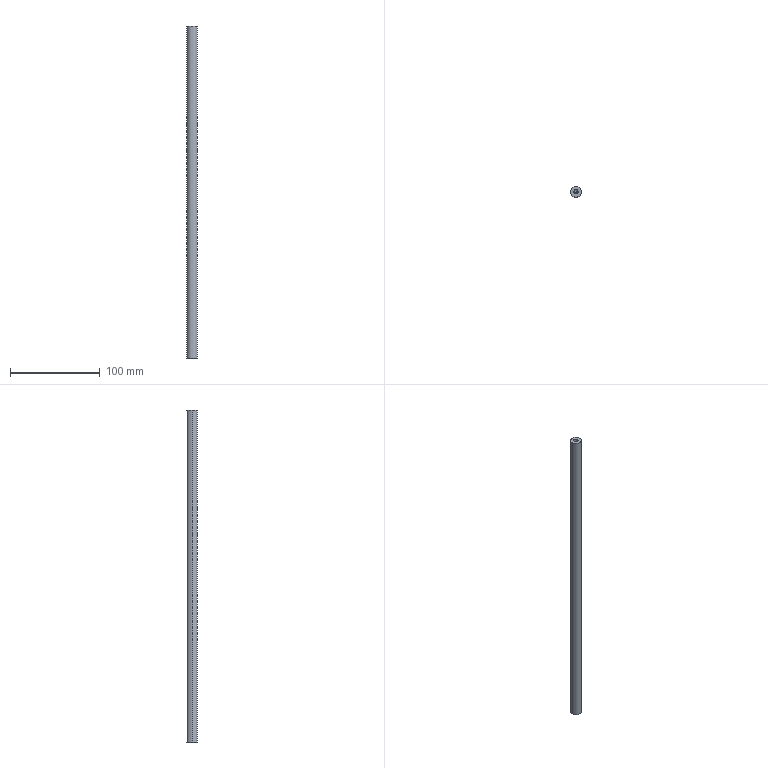Part | STEP file | 602-12-0049 | 1 solid | 12 faces | box 12 x 12 x 370 mm | volume 41119 mm3 | cylinder 6 | cone 4 | plane 2 | commonest cylinder face diameters 5 x4 12 x2
STEP:
#1=CARTESIAN_POINT('',(0.,0.,0.));
#2=DIRECTION('',(0.,0.,1.));
#3=DIRECTION('',(1.,0.,0.));
#4=AXIS2_PLACEMENT_3D('',#1,#2,#3);
#5=CARTESIAN_POINT('',(-2.5,0.,18.));
#6=VERTEX_POINT('',#5);
#7=CARTESIAN_POINT('',(-2.5,0.,0.));
#8=VERTEX_POINT('',#7);
#9=CARTESIAN_POINT('',(-2.5,0.,0.));
#10=DIRECTION('',(0.,0.,-1.));
#11=VECTOR('',#10,1.);
#12=LINE('',#9,#11);
#13=CARTESIAN_POINT('',(0.,0.,0.));
#14=DIRECTION('',(0.,0.,-1.));
#15=DIRECTION('',(-1.,0.,0.));
#16=AXIS2_PLACEMENT_3D('',#13,#14,#15);
#17=CYLINDRICAL_SURFACE('',#16,2.5);
#18=CARTESIAN_POINT('',(6.283,0.));
#19=DIRECTION('',(0.,1.));
#20=VECTOR('',#19,1.);
#21=LINE('',#18,#20);
#22=(GEOMETRIC_REPRESENTATION_CONTEXT(2)PARAMETRIC_REPRESENTATION_CONTEXT()REPRESENTATION_CONTEXT('',''));
#23=DEFINITIONAL_REPRESENTATION('',(#21),#22);
#24=PCURVE('',#17,#23);
#25=CARTESIAN_POINT('',(0.,0.,0.));
#26=DIRECTION('',(0.,0.,-1.));
#27=DIRECTION('',(-1.,0.,0.));
#28=AXIS2_PLACEMENT_3D('',#25,#26,#27);
#29=CYLINDRICAL_SURFACE('',#28,2.5);
#30=CARTESIAN_POINT('',(0.,0.));
#31=DIRECTION('',(0.,1.));
#32=VECTOR('',#31,1.);
#33=LINE('',#30,#32);
#34=(GEOMETRIC_REPRESENTATION_CONTEXT(2)PARAMETRIC_REPRESENTATION_CONTEXT()REPRESENTATION_CONTEXT('',''));
#35=DEFINITIONAL_REPRESENTATION('',(#33),#34);
#36=PCURVE('',#29,#35);
#37=SURFACE_CURVE('',#12,(#24,#36),.PCURVE_S1.);
#38=EDGE_CURVE('',#6,#8,#37,.T.);
#39=ORIENTED_EDGE('',*,*,#38,.T.);
#40=CARTESIAN_POINT('',(2.5,0.,0.));
#41=VERTEX_POINT('',#40);
#42=CARTESIAN_POINT('',(0.,0.,0.));
#43=DIRECTION('',(0.,0.,-1.));
#44=DIRECTION('',(-1.,0.,0.));
#45=AXIS2_PLACEMENT_3D('',#42,#43,#44);
#46=CIRCLE('',#45,2.5);
#47=CARTESIAN_POINT('',(0.,0.));
#48=DIRECTION('',(1.,0.));
#49=VECTOR('',#48,1.);
#50=LINE('',#47,#49);
#51=(GEOMETRIC_REPRESENTATION_CONTEXT(2)PARAMETRIC_REPRESENTATION_CONTEXT()REPRESENTATION_CONTEXT('',''));
#52=DEFINITIONAL_REPRESENTATION('',(#50),#51);
#53=PCURVE('',#17,#52);
#54=CARTESIAN_POINT('',(0.,0.,0.));
#55=DIRECTION('',(0.,0.,1.));
#56=DIRECTION('',(1.,0.,0.));
#57=AXIS2_PLACEMENT_3D('',#54,#55,#56);
#58=PLANE('',#57);
#59=CARTESIAN_POINT('',(-2.5,0.));
#60=CARTESIAN_POINT('',(-2.5,4.33));
#61=CARTESIAN_POINT('',(1.25,2.165));
#62=CARTESIAN_POINT('',(5.,0.));
#63=CARTESIAN_POINT('',(1.25,-2.165));
#64=CARTESIAN_POINT('',(-2.5,-4.33));
#65=CARTESIAN_POINT('',(-2.5,0.));
#66=(BOUNDED_CURVE()B_SPLINE_CURVE(2,(#59,#60,#61,#62,#63,#64,#65),.UNSPECIFIED.,.T.,.F.)B_SPLINE_CURVE_WITH_KNOTS((1,2,2,2,2,1),(-2.094,0.,2.094,4.189,6.283,8.378),.UNSPECIFIED.)CURVE()GEOMETRIC_REPRESENTATION_ITEM()RATIONAL_B_SPLINE_CURVE((1.,0.5,1.,0.5,1.,0.5,1.))REPRESENTATION_ITEM(''));
#67=(GEOMETRIC_REPRESENTATION_CONTEXT(2)PARAMETRIC_REPRESENTATION_CONTEXT()REPRESENTATION_CONTEXT('',''));
#68=DEFINITIONAL_REPRESENTATION('',(#66),#67);
#69=PCURVE('',#58,#68);
#70=SURFACE_CURVE('',#46,(#53,#69),.PCURVE_S1.);
#71=EDGE_CURVE('',#41,#8,#70,.T.);
#72=ORIENTED_EDGE('',*,*,#71,.F.);
#73=CARTESIAN_POINT('',(2.5,0.,18.));
#74=VERTEX_POINT('',#73);
#75=CARTESIAN_POINT('',(2.5,0.,0.));
#76=DIRECTION('',(0.,0.,-1.));
#77=VECTOR('',#76,1.);
#78=LINE('',#75,#77);
#79=CARTESIAN_POINT('',(3.142,0.));
#80=DIRECTION('',(0.,1.));
#81=VECTOR('',#80,1.);
#82=LINE('',#79,#81);
#83=(GEOMETRIC_REPRESENTATION_CONTEXT(2)PARAMETRIC_REPRESENTATION_CONTEXT()REPRESENTATION_CONTEXT('',''));
#84=DEFINITIONAL_REPRESENTATION('',(#82),#83);
#85=PCURVE('',#17,#84);
#86=CARTESIAN_POINT('',(3.142,0.));
#87=DIRECTION('',(0.,1.));
#88=VECTOR('',#87,1.);
#89=LINE('',#86,#88);
#90=(GEOMETRIC_REPRESENTATION_CONTEXT(2)PARAMETRIC_REPRESENTATION_CONTEXT()REPRESENTATION_CONTEXT('',''));
#91=DEFINITIONAL_REPRESENTATION('',(#89),#90);
#92=PCURVE('',#29,#91);
#93=SURFACE_CURVE('',#78,(#85,#92),.PCURVE_S1.);
#94=EDGE_CURVE('',#74,#41,#93,.T.);
#95=ORIENTED_EDGE('',*,*,#94,.F.);
#96=CARTESIAN_POINT('',(0.,0.,18.));
#97=DIRECTION('',(0.,0.,-1.));
#98=DIRECTION('',(-1.,0.,0.));
#99=AXIS2_PLACEMENT_3D('',#96,#97,#98);
#100=CIRCLE('',#99,2.5);
#101=CARTESIAN_POINT('',(0.,-18.));
#102=DIRECTION('',(1.,0.));
#103=VECTOR('',#102,1.);
#104=LINE('',#101,#103);
#105=(GEOMETRIC_REPRESENTATION_CONTEXT(2)PARAMETRIC_REPRESENTATION_CONTEXT()REPRESENTATION_CONTEXT('',''));
#106=DEFINITIONAL_REPRESENTATION('',(#104),#105);
#107=PCURVE('',#17,#106);
#108=CARTESIAN_POINT('',(0.,0.,18.));
#109=DIRECTION('',(0.,0.,-1.));
#110=DIRECTION('',(-1.,0.,0.));
#111=AXIS2_PLACEMENT_3D('',#108,#109,#110);
#112=CONICAL_SURFACE('',#111,2.5,1.03);
#113=CARTESIAN_POINT('',(0.,0.));
#114=DIRECTION('',(1.,0.));
#115=VECTOR('',#114,1.);
#116=LINE('',#113,#115);
#117=(GEOMETRIC_REPRESENTATION_CONTEXT(2)PARAMETRIC_REPRESENTATION_CONTEXT()REPRESENTATION_CONTEXT('',''));
#118=DEFINITIONAL_REPRESENTATION('',(#116),#117);
#119=PCURVE('',#112,#118);
#120=SURFACE_CURVE('',#100,(#107,#119),.PCURVE_S1.);
#121=EDGE_CURVE('',#74,#6,#120,.T.);
#122=ORIENTED_EDGE('',*,*,#121,.T.);
#123=EDGE_LOOP('',(#39,#72,#95,#122));
#124=FACE_BOUND('',#123,.F.);
#125=ADVANCED_FACE('',(#124),#17,.F.);
#126=ORIENTED_EDGE('',*,*,#121,.F.);
#127=CARTESIAN_POINT('',(0.,0.,19.502));
#128=VERTEX_POINT('',#127);
#129=CARTESIAN_POINT('',(2.5,0.,18.));
#130=DIRECTION('',(0.8572,0.,-0.515));
#131=VECTOR('',#130,1.);
#132=LINE('',#129,#131);
#133=CARTESIAN_POINT('',(3.142,-1.502));
#134=CARTESIAN_POINT('',(3.142,-1.479));
#135=CARTESIAN_POINT('',(3.142,-1.434));
#136=CARTESIAN_POINT('',(3.142,-1.366));
#137=CARTESIAN_POINT('',(3.142,-1.297));
#138=CARTESIAN_POINT('',(3.142,-1.229));
#139=CARTESIAN_POINT('',(3.142,-1.161));
#140=CARTESIAN_POINT('',(3.142,-1.092));
#141=CARTESIAN_POINT('',(3.142,-1.024));
#142=CARTESIAN_POINT('',(3.142,-0.9559));
#143=CARTESIAN_POINT('',(3.142,-0.8876));
#144=CARTESIAN_POINT('',(3.142,-0.8194));
#145=CARTESIAN_POINT('',(3.142,-0.7511));
#146=CARTESIAN_POINT('',(3.142,-0.6828));
#147=CARTESIAN_POINT('',(3.142,-0.6145));
#148=CARTESIAN_POINT('',(3.142,-0.5462));
#149=CARTESIAN_POINT('',(3.142,-0.478));
#150=CARTESIAN_POINT('',(3.142,-0.4097));
#151=CARTESIAN_POINT('',(3.142,-0.3414));
#152=CARTESIAN_POINT('',(3.142,-0.2731));
#153=CARTESIAN_POINT('',(3.142,-0.2048));
#154=CARTESIAN_POINT('',(3.142,-0.1366));
#155=CARTESIAN_POINT('',(3.142,-0.06828));
#156=CARTESIAN_POINT('',(3.142,-0.02276));
#157=CARTESIAN_POINT('',(3.142,0.));
#158=B_SPLINE_CURVE_WITH_KNOTS('',3,(#133,#134,#135,#136,#137,#138,#139,#140,#141,#142,#143,#144,#145,#146,#147,#148,#149,#150,#151,#152,#153,#154,#155,#156,#157),.UNSPECIFIED.,.F.,.F.,(4,1,1,1,1,1,1,1,1,1,1,1,1,1,1,1,1,1,1,1,1,1,4),(-2.917,-2.784,-2.651,-2.519,-2.386,-2.254,-2.121,-1.989,-1.856,-1.723,-1.591,-1.458,-1.326,-1.193,-1.061,-0.928,-0.7954,-0.6629,-0.5303,-0.3977,-0.2651,-0.1326,0.),.QUASI_UNIFORM_KNOTS.);
#159=(GEOMETRIC_REPRESENTATION_CONTEXT(2)PARAMETRIC_REPRESENTATION_CONTEXT()REPRESENTATION_CONTEXT('',''));
#160=DEFINITIONAL_REPRESENTATION('',(#158),#159);
#161=PCURVE('',#112,#160);
#162=CARTESIAN_POINT('',(0.,0.,18.));
#163=DIRECTION('',(0.,0.,-1.));
#164=DIRECTION('',(-1.,0.,0.));
#165=AXIS2_PLACEMENT_3D('',#162,#163,#164);
#166=CONICAL_SURFACE('',#165,2.5,1.03);
#167=CARTESIAN_POINT('',(3.142,-1.502));
#168=CARTESIAN_POINT('',(3.142,-1.479));
#169=CARTESIAN_POINT('',(3.142,-1.434));
#170=CARTESIAN_POINT('',(3.142,-1.366));
#171=CARTESIAN_POINT('',(3.142,-1.297));
#172=CARTESIAN_POINT('',(3.142,-1.229));
#173=CARTESIAN_POINT('',(3.142,-1.161));
#174=CARTESIAN_POINT('',(3.142,-1.092));
#175=CARTESIAN_POINT('',(3.142,-1.024));
#176=CARTESIAN_POINT('',(3.142,-0.9559));
#177=CARTESIAN_POINT('',(3.142,-0.8876));
#178=CARTESIAN_POINT('',(3.142,-0.8194));
#179=CARTESIAN_POINT('',(3.142,-0.7511));
#180=CARTESIAN_POINT('',(3.142,-0.6828));
#181=CARTESIAN_POINT('',(3.142,-0.6145));
#182=CARTESIAN_POINT('',(3.142,-0.5462));
#183=CARTESIAN_POINT('',(3.142,-0.478));
#184=CARTESIAN_POINT('',(3.142,-0.4097));
#185=CARTESIAN_POINT('',(3.142,-0.3414));
#186=CARTESIAN_POINT('',(3.142,-0.2731));
#187=CARTESIAN_POINT('',(3.142,-0.2048));
#188=CARTESIAN_POINT('',(3.142,-0.1366));
#189=CARTESIAN_POINT('',(3.142,-0.06828));
#190=CARTESIAN_POINT('',(3.142,-0.02276));
#191=CARTESIAN_POINT('',(3.142,0.));
#192=B_SPLINE_CURVE_WITH_KNOTS('',3,(#167,#168,#169,#170,#171,#172,#173,#174,#175,#176,#177,#178,#179,#180,#181,#182,#183,#184,#185,#186,#187,#188,#189,#190,#191),.UNSPECIFIED.,.F.,.F.,(4,1,1,1,1,1,1,1,1,1,1,1,1,1,1,1,1,1,1,1,1,1,4),(-2.917,-2.784,-2.651,-2.519,-2.386,-2.254,-2.121,-1.989,-1.856,-1.723,-1.591,-1.458,-1.326,-1.193,-1.061,-0.928,-0.7954,-0.6629,-0.5303,-0.3977,-0.2651,-0.1326,0.),.QUASI_UNIFORM_KNOTS.);
#193=(GEOMETRIC_REPRESENTATION_CONTEXT(2)PARAMETRIC_REPRESENTATION_CONTEXT()REPRESENTATION_CONTEXT('',''));
#194=DEFINITIONAL_REPRESENTATION('',(#192),#193);
#195=PCURVE('',#166,#194);
#196=SURFACE_CURVE('',#132,(#161,#195),.PCURVE_S1.);
#197=EDGE_CURVE('',#128,#74,#196,.T.);
#198=ORIENTED_EDGE('',*,*,#197,.F.);
#199=CARTESIAN_POINT('',(-2.5,0.,18.));
#200=DIRECTION('',(-0.8572,0.,-0.515));
#201=VECTOR('',#200,1.);
#202=LINE('',#199,#201);
#203=CARTESIAN_POINT('',(6.283,0.));
#204=DIRECTION('',(0.,1.));
#205=VECTOR('',#204,1.);
#206=LINE('',#203,#205);
#207=(GEOMETRIC_REPRESENTATION_CONTEXT(2)PARAMETRIC_REPRESENTATION_CONTEXT()REPRESENTATION_CONTEXT('',''));
#208=DEFINITIONAL_REPRESENTATION('',(#206),#207);
#209=PCURVE('',#112,#208);
#210=CARTESIAN_POINT('',(0.,0.));
#211=DIRECTION('',(0.,1.));
#212=VECTOR('',#211,1.);
#213=LINE('',#210,#212);
#214=(GEOMETRIC_REPRESENTATION_CONTEXT(2)PARAMETRIC_REPRESENTATION_CONTEXT()REPRESENTATION_CONTEXT('',''));
#215=DEFINITIONAL_REPRESENTATION('',(#213),#214);
#216=PCURVE('',#166,#215);
#217=SURFACE_CURVE('',#202,(#209,#216),.PCURVE_S1.);
#218=EDGE_CURVE('',#128,#6,#217,.T.);
#219=ORIENTED_EDGE('',*,*,#218,.T.);
#220=EDGE_LOOP('',(#126,#198,#219));
#221=FACE_BOUND('',#220,.F.);
#222=ADVANCED_FACE('',(#221),#112,.F.);
#223=CARTESIAN_POINT('',(2.5,0.,352.));
#224=VERTEX_POINT('',#223);
#225=CARTESIAN_POINT('',(2.5,0.,370.));
#226=VERTEX_POINT('',#225);
#227=CARTESIAN_POINT('',(2.5,0.,370.));
#228=DIRECTION('',(0.,0.,1.));
#229=VECTOR('',#228,1.);
#230=LINE('',#227,#229);
#231=CARTESIAN_POINT('',(0.,0.,370.));
#232=DIRECTION('',(0.,0.,1.));
#233=DIRECTION('',(1.,0.,0.));
#234=AXIS2_PLACEMENT_3D('',#231,#232,#233);
#235=CYLINDRICAL_SURFACE('',#234,2.5);
#236=CARTESIAN_POINT('',(6.283,0.));
#237=DIRECTION('',(0.,1.));
#238=VECTOR('',#237,1.);
#239=LINE('',#236,#238);
#240=(GEOMETRIC_REPRESENTATION_CONTEXT(2)PARAMETRIC_REPRESENTATION_CONTEXT()REPRESENTATION_CONTEXT('',''));
#241=DEFINITIONAL_REPRESENTATION('',(#239),#240);
#242=PCURVE('',#235,#241);
#243=CARTESIAN_POINT('',(0.,0.,370.));
#244=DIRECTION('',(0.,0.,1.));
#245=DIRECTION('',(1.,0.,0.));
#246=AXIS2_PLACEMENT_3D('',#243,#244,#245);
#247=CYLINDRICAL_SURFACE('',#246,2.5);
#248=CARTESIAN_POINT('',(0.,0.));
#249=DIRECTION('',(0.,1.));
#250=VECTOR('',#249,1.);
#251=LINE('',#248,#250);
#252=(GEOMETRIC_REPRESENTATION_CONTEXT(2)PARAMETRIC_REPRESENTATION_CONTEXT()REPRESENTATION_CONTEXT('',''));
#253=DEFINITIONAL_REPRESENTATION('',(#251),#252);
#254=PCURVE('',#247,#253);
#255=SURFACE_CURVE('',#230,(#242,#254),.PCURVE_S1.);
#256=EDGE_CURVE('',#224,#226,#255,.T.);
#257=ORIENTED_EDGE('',*,*,#256,.T.);
#258=CARTESIAN_POINT('',(-2.5,0.,370.));
#259=VERTEX_POINT('',#258);
#260=CARTESIAN_POINT('',(0.,0.,370.));
#261=DIRECTION('',(0.,0.,1.));
#262=DIRECTION('',(1.,0.,0.));
#263=AXIS2_PLACEMENT_3D('',#260,#261,#262);
#264=CIRCLE('',#263,2.5);
#265=CARTESIAN_POINT('',(0.,0.));
#266=DIRECTION('',(1.,0.));
#267=VECTOR('',#266,1.);
#268=LINE('',#265,#267);
#269=(GEOMETRIC_REPRESENTATION_CONTEXT(2)PARAMETRIC_REPRESENTATION_CONTEXT()REPRESENTATION_CONTEXT('',''));
#270=DEFINITIONAL_REPRESENTATION('',(#268),#269);
#271=PCURVE('',#235,#270);
#272=CARTESIAN_POINT('',(0.,0.,370.));
#273=DIRECTION('',(0.,0.,1.));
#274=DIRECTION('',(1.,0.,0.));
#275=AXIS2_PLACEMENT_3D('',#272,#273,#274);
#276=PLANE('',#275);
#277=CARTESIAN_POINT('',(0.,0.));
#278=DIRECTION('',(1.,0.));
#279=AXIS2_PLACEMENT_2D('',#277,#278);
#280=CIRCLE('',#279,2.5);
#281=(GEOMETRIC_REPRESENTATION_CONTEXT(2)PARAMETRIC_REPRESENTATION_CONTEXT()REPRESENTATION_CONTEXT('',''));
#282=DEFINITIONAL_REPRESENTATION('',(#280),#281);
#283=PCURVE('',#276,#282);
#284=SURFACE_CURVE('',#264,(#271,#283),.PCURVE_S1.);
#285=EDGE_CURVE('',#259,#226,#284,.T.);
#286=ORIENTED_EDGE('',*,*,#285,.F.);
#287=CARTESIAN_POINT('',(-2.5,0.,352.));
#288=VERTEX_POINT('',#287);
#289=CARTESIAN_POINT('',(-2.5,0.,370.));
#290=DIRECTION('',(0.,0.,1.));
#291=VECTOR('',#290,1.);
#292=LINE('',#289,#291);
#293=CARTESIAN_POINT('',(3.142,0.));
#294=DIRECTION('',(0.,1.));
#295=VECTOR('',#294,1.);
#296=LINE('',#293,#295);
#297=(GEOMETRIC_REPRESENTATION_CONTEXT(2)PARAMETRIC_REPRESENTATION_CONTEXT()REPRESENTATION_CONTEXT('',''));
#298=DEFINITIONAL_REPRESENTATION('',(#296),#297);
#299=PCURVE('',#235,#298);
#300=CARTESIAN_POINT('',(3.142,0.));
#301=DIRECTION('',(0.,1.));
#302=VECTOR('',#301,1.);
#303=LINE('',#300,#302);
#304=(GEOMETRIC_REPRESENTATION_CONTEXT(2)PARAMETRIC_REPRESENTATION_CONTEXT()REPRESENTATION_CONTEXT('',''));
#305=DEFINITIONAL_REPRESENTATION('',(#303),#304);
#306=PCURVE('',#247,#305);
#307=SURFACE_CURVE('',#292,(#299,#306),.PCURVE_S1.);
#308=EDGE_CURVE('',#288,#259,#307,.T.);
#309=ORIENTED_EDGE('',*,*,#308,.F.);
#310=CARTESIAN_POINT('',(0.,0.,352.));
#311=DIRECTION('',(0.,0.,1.));
#312=DIRECTION('',(1.,0.,0.));
#313=AXIS2_PLACEMENT_3D('',#310,#311,#312);
#314=CIRCLE('',#313,2.5);
#315=CARTESIAN_POINT('',(0.,-18.));
#316=DIRECTION('',(1.,0.));
#317=VECTOR('',#316,1.);
#318=LINE('',#315,#317);
#319=(GEOMETRIC_REPRESENTATION_CONTEXT(2)PARAMETRIC_REPRESENTATION_CONTEXT()REPRESENTATION_CONTEXT('',''));
#320=DEFINITIONAL_REPRESENTATION('',(#318),#319);
#321=PCURVE('',#235,#320);
#322=CARTESIAN_POINT('',(0.,0.,352.));
#323=DIRECTION('',(0.,0.,1.));
#324=DIRECTION('',(1.,0.,0.));
#325=AXIS2_PLACEMENT_3D('',#322,#323,#324);
#326=CONICAL_SURFACE('',#325,2.5,1.03);
#327=CARTESIAN_POINT('',(0.,0.));
#328=DIRECTION('',(1.,0.));
#329=VECTOR('',#328,1.);
#330=LINE('',#327,#329);
#331=(GEOMETRIC_REPRESENTATION_CONTEXT(2)PARAMETRIC_REPRESENTATION_CONTEXT()REPRESENTATION_CONTEXT('',''));
#332=DEFINITIONAL_REPRESENTATION('',(#330),#331);
#333=PCURVE('',#326,#332);
#334=SURFACE_CURVE('',#314,(#321,#333),.PCURVE_S1.);
#335=EDGE_CURVE('',#288,#224,#334,.T.);
#336=ORIENTED_EDGE('',*,*,#335,.T.);
#337=EDGE_LOOP('',(#257,#286,#309,#336));
#338=FACE_BOUND('',#337,.F.);
#339=ADVANCED_FACE('',(#338),#235,.F.);
#340=ORIENTED_EDGE('',*,*,#335,.F.);
#341=CARTESIAN_POINT('',(0.,0.,350.498));
#342=VERTEX_POINT('',#341);
#343=CARTESIAN_POINT('',(-2.5,0.,352.));
#344=DIRECTION('',(-0.8572,0.,0.515));
#345=VECTOR('',#344,1.);
#346=LINE('',#343,#345);
#347=CARTESIAN_POINT('',(3.142,-1.502));
#348=CARTESIAN_POINT('',(3.142,-1.479));
#349=CARTESIAN_POINT('',(3.142,-1.434));
#350=CARTESIAN_POINT('',(3.142,-1.366));
#351=CARTESIAN_POINT('',(3.142,-1.297));
#352=CARTESIAN_POINT('',(3.142,-1.229));
#353=CARTESIAN_POINT('',(3.142,-1.161));
#354=CARTESIAN_POINT('',(3.142,-1.092));
#355=CARTESIAN_POINT('',(3.142,-1.024));
#356=CARTESIAN_POINT('',(3.142,-0.9559));
#357=CARTESIAN_POINT('',(3.142,-0.8876));
#358=CARTESIAN_POINT('',(3.142,-0.8194));
#359=CARTESIAN_POINT('',(3.142,-0.7511));
#360=CARTESIAN_POINT('',(3.142,-0.6828));
#361=CARTESIAN_POINT('',(3.142,-0.6145));
#362=CARTESIAN_POINT('',(3.142,-0.5462));
#363=CARTESIAN_POINT('',(3.142,-0.478));
#364=CARTESIAN_POINT('',(3.142,-0.4097));
#365=CARTESIAN_POINT('',(3.142,-0.3414));
#366=CARTESIAN_POINT('',(3.142,-0.2731));
#367=CARTESIAN_POINT('',(3.142,-0.2048));
#368=CARTESIAN_POINT('',(3.142,-0.1366));
#369=CARTESIAN_POINT('',(3.142,-0.06828));
#370=CARTESIAN_POINT('',(3.142,-0.02276));
#371=CARTESIAN_POINT('',(3.142,0.));
#372=B_SPLINE_CURVE_WITH_KNOTS('',3,(#347,#348,#349,#350,#351,#352,#353,#354,#355,#356,#357,#358,#359,#360,#361,#362,#363,#364,#365,#366,#367,#368,#369,#370,#371),.UNSPECIFIED.,.F.,.F.,(4,1,1,1,1,1,1,1,1,1,1,1,1,1,1,1,1,1,1,1,1,1,4),(-2.917,-2.784,-2.651,-2.519,-2.386,-2.254,-2.121,-1.989,-1.856,-1.723,-1.591,-1.458,-1.326,-1.193,-1.061,-0.928,-0.7954,-0.6629,-0.5303,-0.3977,-0.2651,-0.1326,0.),.UNSPECIFIED.);
#373=(GEOMETRIC_REPRESENTATION_CONTEXT(2)PARAMETRIC_REPRESENTATION_CONTEXT()REPRESENTATION_CONTEXT('',''));
#374=DEFINITIONAL_REPRESENTATION('',(#372),#373);
#375=PCURVE('',#326,#374);
#376=CARTESIAN_POINT('',(0.,0.,352.));
#377=DIRECTION('',(0.,0.,1.));
#378=DIRECTION('',(1.,0.,0.));
#379=AXIS2_PLACEMENT_3D('',#376,#377,#378);
#380=CONICAL_SURFACE('',#379,2.5,1.03);
#381=CARTESIAN_POINT('',(3.142,-1.502));
#382=CARTESIAN_POINT('',(3.142,-1.479));
#383=CARTESIAN_POINT('',(3.142,-1.434));
#384=CARTESIAN_POINT('',(3.142,-1.366));
#385=CARTESIAN_POINT('',(3.142,-1.297));
#386=CARTESIAN_POINT('',(3.142,-1.229));
#387=CARTESIAN_POINT('',(3.142,-1.161));
#388=CARTESIAN_POINT('',(3.142,-1.092));
#389=CARTESIAN_POINT('',(3.142,-1.024));
#390=CARTESIAN_POINT('',(3.142,-0.9559));
#391=CARTESIAN_POINT('',(3.142,-0.8876));
#392=CARTESIAN_POINT('',(3.142,-0.8194));
#393=CARTESIAN_POINT('',(3.142,-0.7511));
#394=CARTESIAN_POINT('',(3.142,-0.6828));
#395=CARTESIAN_POINT('',(3.142,-0.6145));
#396=CARTESIAN_POINT('',(3.142,-0.5462));
#397=CARTESIAN_POINT('',(3.142,-0.478));
#398=CARTESIAN_POINT('',(3.142,-0.4097));
#399=CARTESIAN_POINT('',(3.142,-0.3414));
#400=CARTESIAN_POINT('',(3.142,-0.2731));
#401=CARTESIAN_POINT('',(3.142,-0.2048));
#402=CARTESIAN_POINT('',(3.142,-0.1366));
#403=CARTESIAN_POINT('',(3.142,-0.06828));
#404=CARTESIAN_POINT('',(3.142,-0.02276));
#405=CARTESIAN_POINT('',(3.142,0.));
#406=B_SPLINE_CURVE_WITH_KNOTS('',3,(#381,#382,#383,#384,#385,#386,#387,#388,#389,#390,#391,#392,#393,#394,#395,#396,#397,#398,#399,#400,#401,#402,#403,#404,#405),.UNSPECIFIED.,.F.,.F.,(4,1,1,1,1,1,1,1,1,1,1,1,1,1,1,1,1,1,1,1,1,1,4),(-2.917,-2.784,-2.651,-2.519,-2.386,-2.254,-2.121,-1.989,-1.856,-1.723,-1.591,-1.458,-1.326,-1.193,-1.061,-0.928,-0.7954,-0.6629,-0.5303,-0.3977,-0.2651,-0.1326,0.),.UNSPECIFIED.);
#407=(GEOMETRIC_REPRESENTATION_CONTEXT(2)PARAMETRIC_REPRESENTATION_CONTEXT()REPRESENTATION_CONTEXT('',''));
#408=DEFINITIONAL_REPRESENTATION('',(#406),#407);
#409=PCURVE('',#380,#408);
#410=SURFACE_CURVE('',#346,(#375,#409),.PCURVE_S1.);
#411=EDGE_CURVE('',#342,#288,#410,.T.);
#412=ORIENTED_EDGE('',*,*,#411,.F.);
#413=CARTESIAN_POINT('',(2.5,0.,352.));
#414=DIRECTION('',(0.8572,0.,0.515));
#415=VECTOR('',#414,1.);
#416=LINE('',#413,#415);
#417=CARTESIAN_POINT('',(6.283,0.));
#418=DIRECTION('',(0.,1.));
#419=VECTOR('',#418,1.);
#420=LINE('',#417,#419);
#421=(GEOMETRIC_REPRESENTATION_CONTEXT(2)PARAMETRIC_REPRESENTATION_CONTEXT()REPRESENTATION_CONTEXT('',''));
#422=DEFINITIONAL_REPRESENTATION('',(#420),#421);
#423=PCURVE('',#326,#422);
#424=CARTESIAN_POINT('',(0.,0.));
#425=DIRECTION('',(0.,1.));
#426=VECTOR('',#425,1.);
#427=LINE('',#424,#426);
#428=(GEOMETRIC_REPRESENTATION_CONTEXT(2)PARAMETRIC_REPRESENTATION_CONTEXT()REPRESENTATION_CONTEXT('',''));
#429=DEFINITIONAL_REPRESENTATION('',(#427),#428);
#430=PCURVE('',#380,#429);
#431=SURFACE_CURVE('',#416,(#423,#430),.PCURVE_S1.);
#432=EDGE_CURVE('',#342,#224,#431,.T.);
#433=ORIENTED_EDGE('',*,*,#432,.T.);
#434=EDGE_LOOP('',(#340,#412,#433));
#435=FACE_BOUND('',#434,.F.);
#436=ADVANCED_FACE('',(#435),#326,.F.);
#437=CARTESIAN_POINT('',(6.,0.,370.));
#438=VERTEX_POINT('',#437);
#439=CARTESIAN_POINT('',(-6.,0.,370.));
#440=VERTEX_POINT('',#439);
#441=CARTESIAN_POINT('',(0.,0.,370.));
#442=DIRECTION('',(0.,0.,1.));
#443=DIRECTION('',(1.,0.,0.));
#444=AXIS2_PLACEMENT_3D('',#441,#442,#443);
#445=CIRCLE('',#444,6.);
#446=CARTESIAN_POINT('',(0.,0.,370.));
#447=DIRECTION('',(0.,0.,-1.));
#448=DIRECTION('',(-1.,0.,0.));
#449=AXIS2_PLACEMENT_3D('',#446,#447,#448);
#450=CYLINDRICAL_SURFACE('',#449,6.);
#451=CARTESIAN_POINT('',(3.142,0.));
#452=DIRECTION('',(-1.,0.));
#453=VECTOR('',#452,1.);
#454=LINE('',#451,#453);
#455=(GEOMETRIC_REPRESENTATION_CONTEXT(2)PARAMETRIC_REPRESENTATION_CONTEXT()REPRESENTATION_CONTEXT('',''));
#456=DEFINITIONAL_REPRESENTATION('',(#454),#455);
#457=PCURVE('',#450,#456);
#458=CARTESIAN_POINT('',(0.,0.));
#459=DIRECTION('',(1.,0.));
#460=AXIS2_PLACEMENT_2D('',#458,#459);
#461=CIRCLE('',#460,6.);
#462=(GEOMETRIC_REPRESENTATION_CONTEXT(2)PARAMETRIC_REPRESENTATION_CONTEXT()REPRESENTATION_CONTEXT('',''));
#463=DEFINITIONAL_REPRESENTATION('',(#461),#462);
#464=PCURVE('',#276,#463);
#465=SURFACE_CURVE('',#445,(#457,#464),.PCURVE_S1.);
#466=EDGE_CURVE('',#438,#440,#465,.T.);
#467=ORIENTED_EDGE('',*,*,#466,.F.);
#468=CARTESIAN_POINT('',(6.,0.,0.));
#469=VERTEX_POINT('',#468);
#470=CARTESIAN_POINT('',(6.,0.,370.));
#471=DIRECTION('',(0.,0.,-1.));
#472=VECTOR('',#471,1.);
#473=LINE('',#470,#472);
#474=CARTESIAN_POINT('',(3.142,0.));
#475=DIRECTION('',(0.,1.));
#476=VECTOR('',#475,1.);
#477=LINE('',#474,#476);
#478=(GEOMETRIC_REPRESENTATION_CONTEXT(2)PARAMETRIC_REPRESENTATION_CONTEXT()REPRESENTATION_CONTEXT('',''));
#479=DEFINITIONAL_REPRESENTATION('',(#477),#478);
#480=PCURVE('',#450,#479);
#481=CARTESIAN_POINT('',(0.,0.,370.));
#482=DIRECTION('',(0.,0.,-1.));
#483=DIRECTION('',(-1.,0.,0.));
#484=AXIS2_PLACEMENT_3D('',#481,#482,#483);
#485=CYLINDRICAL_SURFACE('',#484,6.);
#486=CARTESIAN_POINT('',(3.142,0.));
#487=DIRECTION('',(0.,1.));
#488=VECTOR('',#487,1.);
#489=LINE('',#486,#488);
#490=(GEOMETRIC_REPRESENTATION_CONTEXT(2)PARAMETRIC_REPRESENTATION_CONTEXT()REPRESENTATION_CONTEXT('',''));
#491=DEFINITIONAL_REPRESENTATION('',(#489),#490);
#492=PCURVE('',#485,#491);
#493=SURFACE_CURVE('',#473,(#480,#492),.PCURVE_S1.);
#494=EDGE_CURVE('',#438,#469,#493,.T.);
#495=ORIENTED_EDGE('',*,*,#494,.T.);
#496=CARTESIAN_POINT('',(-6.,0.,0.));
#497=VERTEX_POINT('',#496);
#498=CARTESIAN_POINT('',(0.,0.,0.));
#499=DIRECTION('',(0.,0.,1.));
#500=DIRECTION('',(1.,0.,0.));
#501=AXIS2_PLACEMENT_3D('',#498,#499,#500);
#502=CIRCLE('',#501,6.);
#503=CARTESIAN_POINT('',(3.142,370.));
#504=DIRECTION('',(-1.,0.));
#505=VECTOR('',#504,1.);
#506=LINE('',#503,#505);
#507=(GEOMETRIC_REPRESENTATION_CONTEXT(2)PARAMETRIC_REPRESENTATION_CONTEXT()REPRESENTATION_CONTEXT('',''));
#508=DEFINITIONAL_REPRESENTATION('',(#506),#507);
#509=PCURVE('',#450,#508);
#510=CARTESIAN_POINT('',(0.,0.));
#511=DIRECTION('',(1.,0.));
#512=AXIS2_PLACEMENT_2D('',#510,#511);
#513=CIRCLE('',#512,6.);
#514=(GEOMETRIC_REPRESENTATION_CONTEXT(2)PARAMETRIC_REPRESENTATION_CONTEXT()REPRESENTATION_CONTEXT('',''));
#515=DEFINITIONAL_REPRESENTATION('',(#513),#514);
#516=PCURVE('',#58,#515);
#517=SURFACE_CURVE('',#502,(#509,#516),.PCURVE_S1.);
#518=EDGE_CURVE('',#469,#497,#517,.T.);
#519=ORIENTED_EDGE('',*,*,#518,.T.);
#520=CARTESIAN_POINT('',(-6.,0.,370.));
#521=DIRECTION('',(0.,0.,-1.));
#522=VECTOR('',#521,1.);
#523=LINE('',#520,#522);
#524=CARTESIAN_POINT('',(0.,0.));
#525=DIRECTION('',(0.,1.));
#526=VECTOR('',#525,1.);
#527=LINE('',#524,#526);
#528=(GEOMETRIC_REPRESENTATION_CONTEXT(2)PARAMETRIC_REPRESENTATION_CONTEXT()REPRESENTATION_CONTEXT('',''));
#529=DEFINITIONAL_REPRESENTATION('',(#527),#528);
#530=PCURVE('',#450,#529);
#531=CARTESIAN_POINT('',(6.283,0.));
#532=DIRECTION('',(0.,1.));
#533=VECTOR('',#532,1.);
#534=LINE('',#531,#533);
#535=(GEOMETRIC_REPRESENTATION_CONTEXT(2)PARAMETRIC_REPRESENTATION_CONTEXT()REPRESENTATION_CONTEXT('',''));
#536=DEFINITIONAL_REPRESENTATION('',(#534),#535);
#537=PCURVE('',#485,#536);
#538=SURFACE_CURVE('',#523,(#530,#537),.PCURVE_S1.);
#539=EDGE_CURVE('',#440,#497,#538,.T.);
#540=ORIENTED_EDGE('',*,*,#539,.F.);
#541=EDGE_LOOP('',(#467,#495,#519,#540));
#542=FACE_BOUND('',#541,.T.);
#543=ADVANCED_FACE('',(#542),#450,.T.);
#544=ORIENTED_EDGE('',*,*,#494,.F.);
#545=CARTESIAN_POINT('',(0.,0.,370.));
#546=DIRECTION('',(0.,0.,1.));
#547=DIRECTION('',(1.,0.,0.));
#548=AXIS2_PLACEMENT_3D('',#545,#546,#547);
#549=CIRCLE('',#548,6.);
#550=CARTESIAN_POINT('',(9.425,0.));
#551=DIRECTION('',(-1.,0.));
#552=VECTOR('',#551,1.);
#553=LINE('',#550,#552);
#554=(GEOMETRIC_REPRESENTATION_CONTEXT(2)PARAMETRIC_REPRESENTATION_CONTEXT()REPRESENTATION_CONTEXT('',''));
#555=DEFINITIONAL_REPRESENTATION('',(#553),#554);
#556=PCURVE('',#485,#555);
#557=CARTESIAN_POINT('',(0.,0.));
#558=DIRECTION('',(1.,0.));
#559=AXIS2_PLACEMENT_2D('',#557,#558);
#560=CIRCLE('',#559,6.);
#561=(GEOMETRIC_REPRESENTATION_CONTEXT(2)PARAMETRIC_REPRESENTATION_CONTEXT()REPRESENTATION_CONTEXT('',''));
#562=DEFINITIONAL_REPRESENTATION('',(#560),#561);
#563=PCURVE('',#276,#562);
#564=SURFACE_CURVE('',#549,(#556,#563),.PCURVE_S1.);
#565=EDGE_CURVE('',#440,#438,#564,.T.);
#566=ORIENTED_EDGE('',*,*,#565,.F.);
#567=ORIENTED_EDGE('',*,*,#539,.T.);
#568=CARTESIAN_POINT('',(0.,0.,0.));
#569=DIRECTION('',(0.,0.,1.));
#570=DIRECTION('',(1.,0.,0.));
#571=AXIS2_PLACEMENT_3D('',#568,#569,#570);
#572=CIRCLE('',#571,6.);
#573=CARTESIAN_POINT('',(9.425,370.));
#574=DIRECTION('',(-1.,0.));
#575=VECTOR('',#574,1.);
#576=LINE('',#573,#575);
#577=(GEOMETRIC_REPRESENTATION_CONTEXT(2)PARAMETRIC_REPRESENTATION_CONTEXT()REPRESENTATION_CONTEXT('',''));
#578=DEFINITIONAL_REPRESENTATION('',(#576),#577);
#579=PCURVE('',#485,#578);
#580=CARTESIAN_POINT('',(0.,0.));
#581=DIRECTION('',(1.,0.));
#582=AXIS2_PLACEMENT_2D('',#580,#581);
#583=CIRCLE('',#582,6.);
#584=(GEOMETRIC_REPRESENTATION_CONTEXT(2)PARAMETRIC_REPRESENTATION_CONTEXT()REPRESENTATION_CONTEXT('',''));
#585=DEFINITIONAL_REPRESENTATION('',(#583),#584);
#586=PCURVE('',#58,#585);
#587=SURFACE_CURVE('',#572,(#579,#586),.PCURVE_S1.);
#588=EDGE_CURVE('',#497,#469,#587,.T.);
#589=ORIENTED_EDGE('',*,*,#588,.T.);
#590=EDGE_LOOP('',(#544,#566,#567,#589));
#591=FACE_BOUND('',#590,.T.);
#592=ADVANCED_FACE('',(#591),#485,.T.);
#593=CARTESIAN_POINT('',(0.,0.,370.));
#594=DIRECTION('',(0.,0.,1.));
#595=DIRECTION('',(1.,0.,0.));
#596=AXIS2_PLACEMENT_3D('',#593,#594,#595);
#597=CIRCLE('',#596,2.5);
#598=CARTESIAN_POINT('',(0.,0.));
#599=DIRECTION('',(1.,0.));
#600=AXIS2_PLACEMENT_2D('',#598,#599);
#601=CIRCLE('',#600,2.5);
#602=(GEOMETRIC_REPRESENTATION_CONTEXT(2)PARAMETRIC_REPRESENTATION_CONTEXT()REPRESENTATION_CONTEXT('',''));
#603=DEFINITIONAL_REPRESENTATION('',(#601),#602);
#604=PCURVE('',#276,#603);
#605=CARTESIAN_POINT('',(0.,0.));
#606=DIRECTION('',(1.,0.));
#607=VECTOR('',#606,1.);
#608=LINE('',#605,#607);
#609=(GEOMETRIC_REPRESENTATION_CONTEXT(2)PARAMETRIC_REPRESENTATION_CONTEXT()REPRESENTATION_CONTEXT('',''));
#610=DEFINITIONAL_REPRESENTATION('',(#608),#609);
#611=PCURVE('',#247,#610);
#612=SURFACE_CURVE('',#597,(#604,#611),.PCURVE_S1.);
#613=EDGE_CURVE('',#226,#259,#612,.T.);
#614=ORIENTED_EDGE('',*,*,#613,.F.);
#615=ORIENTED_EDGE('',*,*,#285,.F.);
#616=EDGE_LOOP('',(#614,#615));
#617=FACE_BOUND('',#616,.T.);
#618=ORIENTED_EDGE('',*,*,#565,.T.);
#619=ORIENTED_EDGE('',*,*,#466,.T.);
#620=EDGE_LOOP('',(#618,#619));
#621=FACE_BOUND('',#620,.T.);
#622=ADVANCED_FACE('',(#617,#621),#276,.T.);
#623=CARTESIAN_POINT('',(0.,0.,0.));
#624=DIRECTION('',(0.,0.,-1.));
#625=DIRECTION('',(-1.,0.,0.));
#626=AXIS2_PLACEMENT_3D('',#623,#624,#625);
#627=CIRCLE('',#626,2.5);
#628=CARTESIAN_POINT('',(-2.5,0.));
#629=CARTESIAN_POINT('',(-2.5,4.33));
#630=CARTESIAN_POINT('',(1.25,2.165));
#631=CARTESIAN_POINT('',(5.,0.));
#632=CARTESIAN_POINT('',(1.25,-2.165));
#633=CARTESIAN_POINT('',(-2.5,-4.33));
#634=CARTESIAN_POINT('',(-2.5,0.));
#635=(BOUNDED_CURVE()B_SPLINE_CURVE(2,(#628,#629,#630,#631,#632,#633,#634),.UNSPECIFIED.,.T.,.F.)B_SPLINE_CURVE_WITH_KNOTS((1,2,2,2,2,1),(-2.094,0.,2.094,4.189,6.283,8.378),.UNSPECIFIED.)CURVE()GEOMETRIC_REPRESENTATION_ITEM()RATIONAL_B_SPLINE_CURVE((1.,0.5,1.,0.5,1.,0.5,1.))REPRESENTATION_ITEM(''));
#636=(GEOMETRIC_REPRESENTATION_CONTEXT(2)PARAMETRIC_REPRESENTATION_CONTEXT()REPRESENTATION_CONTEXT('',''));
#637=DEFINITIONAL_REPRESENTATION('',(#635),#636);
#638=PCURVE('',#58,#637);
#639=CARTESIAN_POINT('',(0.,0.));
#640=DIRECTION('',(1.,0.));
#641=VECTOR('',#640,1.);
#642=LINE('',#639,#641);
#643=(GEOMETRIC_REPRESENTATION_CONTEXT(2)PARAMETRIC_REPRESENTATION_CONTEXT()REPRESENTATION_CONTEXT('',''));
#644=DEFINITIONAL_REPRESENTATION('',(#642),#643);
#645=PCURVE('',#29,#644);
#646=SURFACE_CURVE('',#627,(#638,#645),.PCURVE_S1.);
#647=EDGE_CURVE('',#8,#41,#646,.T.);
#648=ORIENTED_EDGE('',*,*,#647,.F.);
#649=ORIENTED_EDGE('',*,*,#71,.F.);
#650=EDGE_LOOP('',(#648,#649));
#651=FACE_BOUND('',#650,.T.);
#652=ORIENTED_EDGE('',*,*,#588,.F.);
#653=ORIENTED_EDGE('',*,*,#518,.F.);
#654=EDGE_LOOP('',(#652,#653));
#655=FACE_BOUND('',#654,.T.);
#656=ADVANCED_FACE('',(#651,#655),#58,.F.);
#657=CARTESIAN_POINT('',(0.,0.,352.));
#658=DIRECTION('',(0.,0.,1.));
#659=DIRECTION('',(1.,0.,0.));
#660=AXIS2_PLACEMENT_3D('',#657,#658,#659);
#661=CIRCLE('',#660,2.5);
#662=CARTESIAN_POINT('',(0.,0.));
#663=DIRECTION('',(1.,0.));
#664=VECTOR('',#663,1.);
#665=LINE('',#662,#664);
#666=(GEOMETRIC_REPRESENTATION_CONTEXT(2)PARAMETRIC_REPRESENTATION_CONTEXT()REPRESENTATION_CONTEXT('',''));
#667=DEFINITIONAL_REPRESENTATION('',(#665),#666);
#668=PCURVE('',#380,#667);
#669=CARTESIAN_POINT('',(0.,-18.));
#670=DIRECTION('',(1.,0.));
#671=VECTOR('',#670,1.);
#672=LINE('',#669,#671);
#673=(GEOMETRIC_REPRESENTATION_CONTEXT(2)PARAMETRIC_REPRESENTATION_CONTEXT()REPRESENTATION_CONTEXT('',''));
#674=DEFINITIONAL_REPRESENTATION('',(#672),#673);
#675=PCURVE('',#247,#674);
#676=SURFACE_CURVE('',#661,(#668,#675),.PCURVE_S1.);
#677=EDGE_CURVE('',#224,#288,#676,.T.);
#678=ORIENTED_EDGE('',*,*,#677,.F.);
#679=ORIENTED_EDGE('',*,*,#432,.F.);
#680=ORIENTED_EDGE('',*,*,#411,.T.);
#681=EDGE_LOOP('',(#678,#679,#680));
#682=FACE_BOUND('',#681,.F.);
#683=ADVANCED_FACE('',(#682),#380,.F.);
#684=ORIENTED_EDGE('',*,*,#613,.F.);
#685=ORIENTED_EDGE('',*,*,#256,.F.);
#686=ORIENTED_EDGE('',*,*,#677,.T.);
#687=ORIENTED_EDGE('',*,*,#308,.T.);
#688=EDGE_LOOP('',(#684,#685,#686,#687));
#689=FACE_BOUND('',#688,.F.);
#690=ADVANCED_FACE('',(#689),#247,.F.);
#691=CARTESIAN_POINT('',(0.,0.,18.));
#692=DIRECTION('',(0.,0.,-1.));
#693=DIRECTION('',(-1.,0.,0.));
#694=AXIS2_PLACEMENT_3D('',#691,#692,#693);
#695=CIRCLE('',#694,2.5);
#696=CARTESIAN_POINT('',(0.,0.));
#697=DIRECTION('',(1.,0.));
#698=VECTOR('',#697,1.);
#699=LINE('',#696,#698);
#700=(GEOMETRIC_REPRESENTATION_CONTEXT(2)PARAMETRIC_REPRESENTATION_CONTEXT()REPRESENTATION_CONTEXT('',''));
#701=DEFINITIONAL_REPRESENTATION('',(#699),#700);
#702=PCURVE('',#166,#701);
#703=CARTESIAN_POINT('',(0.,-18.));
#704=DIRECTION('',(1.,0.));
#705=VECTOR('',#704,1.);
#706=LINE('',#703,#705);
#707=(GEOMETRIC_REPRESENTATION_CONTEXT(2)PARAMETRIC_REPRESENTATION_CONTEXT()REPRESENTATION_CONTEXT('',''));
#708=DEFINITIONAL_REPRESENTATION('',(#706),#707);
#709=PCURVE('',#29,#708);
#710=SURFACE_CURVE('',#695,(#702,#709),.PCURVE_S1.);
#711=EDGE_CURVE('',#6,#74,#710,.T.);
#712=ORIENTED_EDGE('',*,*,#711,.F.);
#713=ORIENTED_EDGE('',*,*,#218,.F.);
#714=ORIENTED_EDGE('',*,*,#197,.T.);
#715=EDGE_LOOP('',(#712,#713,#714));
#716=FACE_BOUND('',#715,.F.);
#717=ADVANCED_FACE('',(#716),#166,.F.);
#718=ORIENTED_EDGE('',*,*,#647,.F.);
#719=ORIENTED_EDGE('',*,*,#38,.F.);
#720=ORIENTED_EDGE('',*,*,#711,.T.);
#721=ORIENTED_EDGE('',*,*,#94,.T.);
#722=EDGE_LOOP('',(#718,#719,#720,#721));
#723=FACE_BOUND('',#722,.F.);
#724=ADVANCED_FACE('',(#723),#29,.F.);
#725=CLOSED_SHELL('',(#125,#222,#339,#436,#543,#592,#622,#656,#683,#690,#717,#724));
#726=MANIFOLD_SOLID_BREP('',#725);
#727=(LENGTH_UNIT()NAMED_UNIT(*)SI_UNIT(.MILLI.,.METRE.));
#728=UNCERTAINTY_MEASURE_WITH_UNIT(LENGTH_MEASURE(0.0000001),#727,'','');
#729=(NAMED_UNIT(*)PLANE_ANGLE_UNIT()SI_UNIT($,.RADIAN.));
#730=(NAMED_UNIT(*)SI_UNIT($,.STERADIAN.)SOLID_ANGLE_UNIT());
#731=(GEOMETRIC_REPRESENTATION_CONTEXT(3)GLOBAL_UNCERTAINTY_ASSIGNED_CONTEXT((#728))GLOBAL_UNIT_ASSIGNED_CONTEXT((#727,#729,#730))REPRESENTATION_CONTEXT('',''));
#732=ADVANCED_BREP_SHAPE_REPRESENTATION('',(#4,#726),#731);